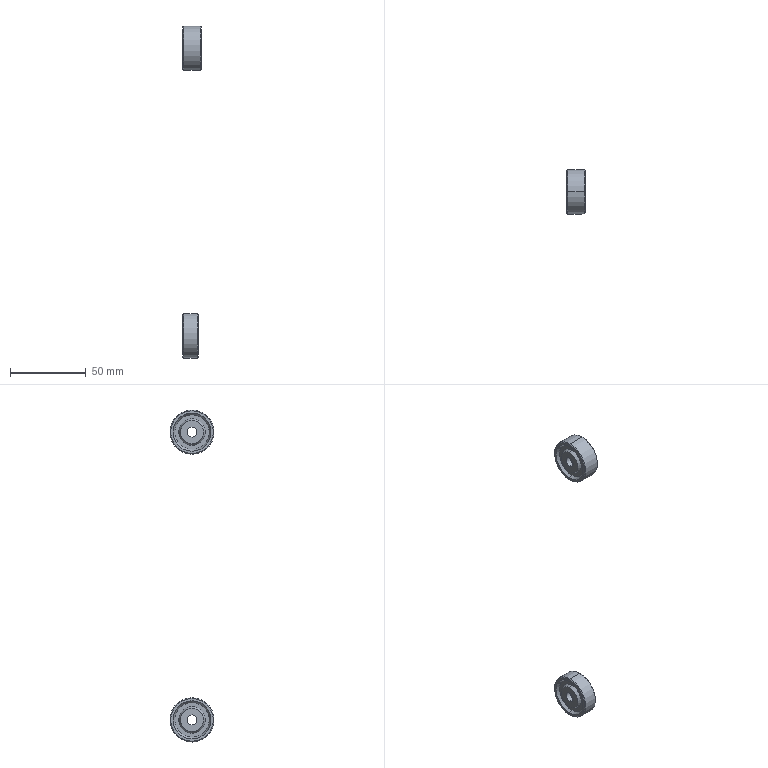Part | STEP file | INSULATION DISC | 2 solids | 50 faces | box 12 x 29.2 x 219.2 mm | volume 11077 mm3 | cone 24 | plane 14 | cylinder 12 | commonest cylinder face diameters 6.5 x4 11 x4 29.2 x4